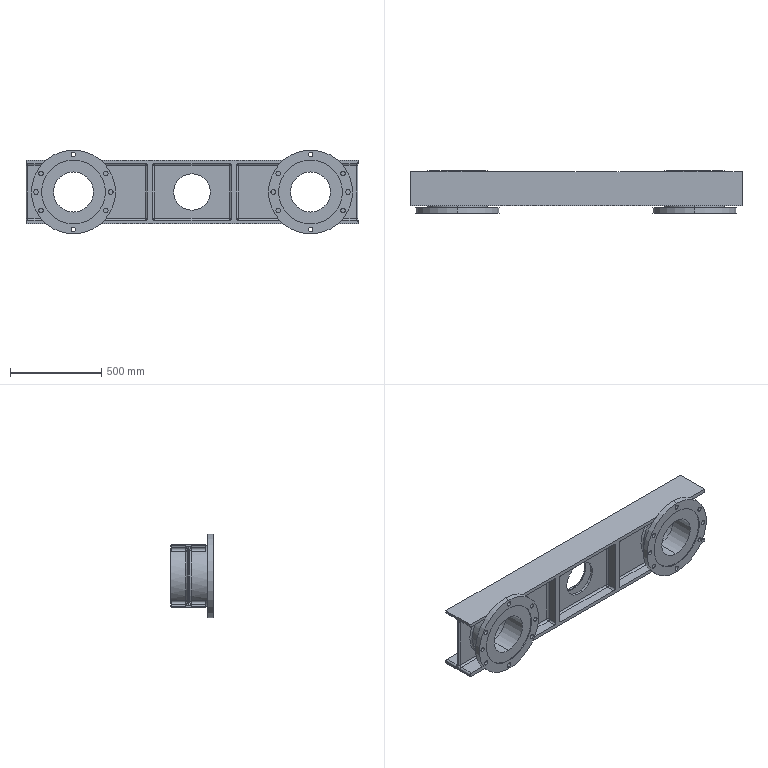Part | STEP file | Bearing housing | 1 solid | 268 faces | box 1820 x 234 x 460 mm | volume 47518256 mm3 | cylinder 146 | plane 72 | sphere 32 | torus 18 | commonest cylinder face diameters 20 x84 25 x32 330 x10 200 x4 220 x4 270 x4